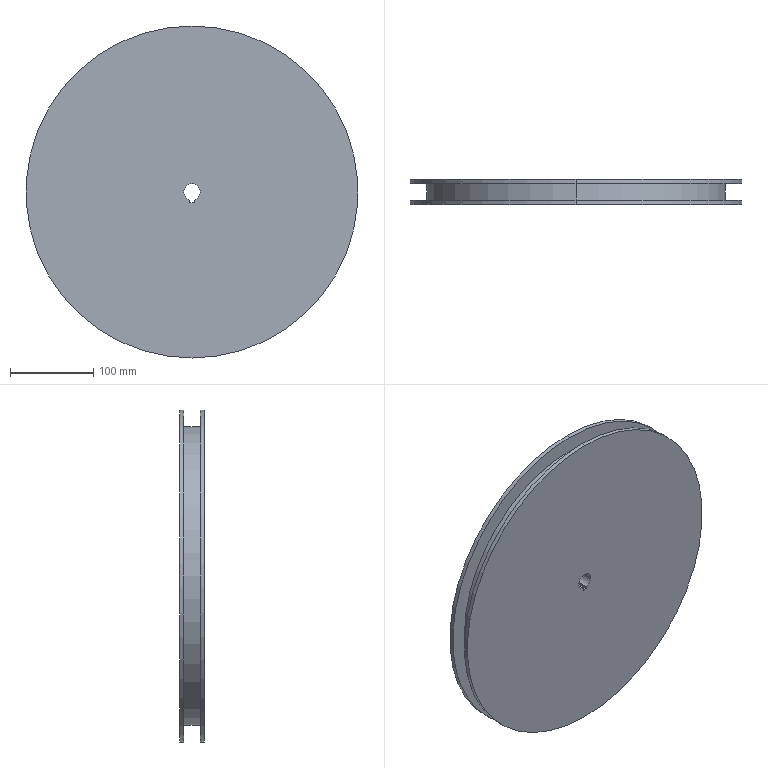Part | SolidWorks | features ICE 1, Revolution 1 | 1 solid | 15 faces | box 400 x 30 x 400 mm | volume 3282546 mm3 | cylinder 8 | plane 7 | commonest cylinder face diameters 400 x4 20 x2 360 x2
STEP:
#1=CARTESIAN_POINT('',(0.,-5.,200.));
#2=VERTEX_POINT('',#1);
#3=CARTESIAN_POINT('',(0.,-5.,-200.));
#4=VERTEX_POINT('',#3);
#5=CARTESIAN_POINT('',(0.,-5.,0.));
#6=DIRECTION('',(0.,1.,0.));
#7=DIRECTION('',(0.,0.,1.));
#8=AXIS2_PLACEMENT_3D('',#5,#6,#7);
#9=CIRCLE('',#8,200.);
#10=EDGE_CURVE('',#2,#4,#9,.T.);
#11=ORIENTED_EDGE('',*,*,#10,.T.);
#12=CARTESIAN_POINT('',(0.,0.,-200.));
#13=VERTEX_POINT('',#12);
#14=CARTESIAN_POINT('',(0.,76.759,-200.));
#15=DIRECTION('',(0.,1.,0.));
#16=VECTOR('',#15,1000.);
#17=LINE('',#14,#16);
#18=EDGE_CURVE('',#4,#13,#17,.T.);
#19=ORIENTED_EDGE('',*,*,#18,.T.);
#20=CARTESIAN_POINT('',(0.,0.,200.));
#21=VERTEX_POINT('',#20);
#22=CARTESIAN_POINT('',(0.,0.,0.));
#23=DIRECTION('',(0.,1.,0.));
#24=DIRECTION('',(0.,0.,1.));
#25=AXIS2_PLACEMENT_3D('',#22,#23,#24);
#26=CIRCLE('',#25,200.);
#27=EDGE_CURVE('',#21,#13,#26,.T.);
#28=ORIENTED_EDGE('',*,*,#27,.F.);
#29=CARTESIAN_POINT('',(0.,76.759,200.));
#30=DIRECTION('',(0.,1.,0.));
#31=VECTOR('',#30,1000.);
#32=LINE('',#29,#31);
#33=EDGE_CURVE('',#2,#21,#32,.T.);
#34=ORIENTED_EDGE('',*,*,#33,.F.);
#35=EDGE_LOOP('',(#11,#19,#28,#34));
#36=FACE_OUTER_BOUND('',#35,.T.);
#37=CARTESIAN_POINT('',(0.,76.759,0.));
#38=DIRECTION('',(0.,1.,0.));
#39=DIRECTION('',(0.,0.,1.));
#40=AXIS2_PLACEMENT_3D('',#37,#38,#39);
#41=CYLINDRICAL_SURFACE('',#40,200.);
#42=ADVANCED_FACE('',(#36),#41,.T.);
#43=CARTESIAN_POINT('',(0.,-25.,180.));
#44=VERTEX_POINT('',#43);
#45=CARTESIAN_POINT('',(0.,-25.,-180.));
#46=VERTEX_POINT('',#45);
#47=CARTESIAN_POINT('',(0.,-25.,0.));
#48=DIRECTION('',(0.,1.,0.));
#49=DIRECTION('',(0.,0.,1.));
#50=AXIS2_PLACEMENT_3D('',#47,#48,#49);
#51=CIRCLE('',#50,180.);
#52=EDGE_CURVE('',#44,#46,#51,.T.);
#53=ORIENTED_EDGE('',*,*,#52,.T.);
#54=CARTESIAN_POINT('',(0.,-5.,-180.));
#55=VERTEX_POINT('',#54);
#56=CARTESIAN_POINT('',(0.,76.759,-180.));
#57=DIRECTION('',(0.,1.,0.));
#58=VECTOR('',#57,1000.);
#59=LINE('',#56,#58);
#60=EDGE_CURVE('',#46,#55,#59,.T.);
#61=ORIENTED_EDGE('',*,*,#60,.T.);
#62=CARTESIAN_POINT('',(0.,-5.,180.));
#63=VERTEX_POINT('',#62);
#64=CARTESIAN_POINT('',(0.,-5.,0.));
#65=DIRECTION('',(0.,1.,0.));
#66=DIRECTION('',(0.,0.,1.));
#67=AXIS2_PLACEMENT_3D('',#64,#65,#66);
#68=CIRCLE('',#67,180.);
#69=EDGE_CURVE('',#63,#55,#68,.T.);
#70=ORIENTED_EDGE('',*,*,#69,.F.);
#71=CARTESIAN_POINT('',(0.,76.759,180.));
#72=DIRECTION('',(0.,1.,0.));
#73=VECTOR('',#72,1000.);
#74=LINE('',#71,#73);
#75=EDGE_CURVE('',#44,#63,#74,.T.);
#76=ORIENTED_EDGE('',*,*,#75,.F.);
#77=EDGE_LOOP('',(#53,#61,#70,#76));
#78=FACE_OUTER_BOUND('',#77,.T.);
#79=CARTESIAN_POINT('',(0.,76.759,0.));
#80=DIRECTION('',(0.,1.,0.));
#81=DIRECTION('',(0.,0.,1.));
#82=AXIS2_PLACEMENT_3D('',#79,#80,#81);
#83=CYLINDRICAL_SURFACE('',#82,180.);
#84=ADVANCED_FACE('',(#78),#83,.T.);
#85=CARTESIAN_POINT('',(0.,-30.,200.));
#86=VERTEX_POINT('',#85);
#87=CARTESIAN_POINT('',(0.,-30.,-200.));
#88=VERTEX_POINT('',#87);
#89=CARTESIAN_POINT('',(0.,-30.,0.));
#90=DIRECTION('',(0.,1.,0.));
#91=DIRECTION('',(0.,0.,1.));
#92=AXIS2_PLACEMENT_3D('',#89,#90,#91);
#93=CIRCLE('',#92,200.);
#94=EDGE_CURVE('',#86,#88,#93,.T.);
#95=ORIENTED_EDGE('',*,*,#94,.T.);
#96=CARTESIAN_POINT('',(0.,-25.,-200.));
#97=VERTEX_POINT('',#96);
#98=CARTESIAN_POINT('',(0.,76.759,-200.));
#99=DIRECTION('',(0.,1.,0.));
#100=VECTOR('',#99,1000.);
#101=LINE('',#98,#100);
#102=EDGE_CURVE('',#88,#97,#101,.T.);
#103=ORIENTED_EDGE('',*,*,#102,.T.);
#104=CARTESIAN_POINT('',(0.,-25.,200.));
#105=VERTEX_POINT('',#104);
#106=CARTESIAN_POINT('',(0.,-25.,0.));
#107=DIRECTION('',(0.,1.,0.));
#108=DIRECTION('',(0.,0.,1.));
#109=AXIS2_PLACEMENT_3D('',#106,#107,#108);
#110=CIRCLE('',#109,200.);
#111=EDGE_CURVE('',#105,#97,#110,.T.);
#112=ORIENTED_EDGE('',*,*,#111,.F.);
#113=CARTESIAN_POINT('',(0.,76.759,200.));
#114=DIRECTION('',(0.,1.,0.));
#115=VECTOR('',#114,1000.);
#116=LINE('',#113,#115);
#117=EDGE_CURVE('',#86,#105,#116,.T.);
#118=ORIENTED_EDGE('',*,*,#117,.F.);
#119=EDGE_LOOP('',(#95,#103,#112,#118));
#120=FACE_OUTER_BOUND('',#119,.T.);
#121=CARTESIAN_POINT('',(0.,76.759,0.));
#122=DIRECTION('',(0.,1.,0.));
#123=DIRECTION('',(0.,0.,1.));
#124=AXIS2_PLACEMENT_3D('',#121,#122,#123);
#125=CYLINDRICAL_SURFACE('',#124,200.);
#126=ADVANCED_FACE('',(#120),#125,.T.);
#127=CARTESIAN_POINT('',(0.,-30.,10.));
#128=VERTEX_POINT('',#127);
#129=CARTESIAN_POINT('',(2.5,-30.,-9.682));
#130=VERTEX_POINT('',#129);
#131=CARTESIAN_POINT('',(0.,-30.,0.));
#132=DIRECTION('',(0.,1.,0.));
#133=DIRECTION('',(0.,0.,1.));
#134=AXIS2_PLACEMENT_3D('',#131,#132,#133);
#135=CIRCLE('',#134,10.);
#136=EDGE_CURVE('',#128,#130,#135,.T.);
#137=ORIENTED_EDGE('',*,*,#136,.F.);
#138=CARTESIAN_POINT('',(0.,0.,10.));
#139=VERTEX_POINT('',#138);
#140=CARTESIAN_POINT('',(0.,76.759,10.));
#141=DIRECTION('',(0.,1.,0.));
#142=VECTOR('',#141,1000.);
#143=LINE('',#140,#142);
#144=EDGE_CURVE('',#128,#139,#143,.T.);
#145=ORIENTED_EDGE('',*,*,#144,.T.);
#146=CARTESIAN_POINT('',(2.5,0.,-9.682));
#147=VERTEX_POINT('',#146);
#148=CARTESIAN_POINT('',(0.,0.,0.));
#149=DIRECTION('',(0.,1.,0.));
#150=DIRECTION('',(0.,0.,1.));
#151=AXIS2_PLACEMENT_3D('',#148,#149,#150);
#152=CIRCLE('',#151,10.);
#153=EDGE_CURVE('',#139,#147,#152,.T.);
#154=ORIENTED_EDGE('',*,*,#153,.T.);
#155=CARTESIAN_POINT('',(2.5,-30.,-9.682));
#156=DIRECTION('',(0.,1.,0.));
#157=VECTOR('',#156,1000.);
#158=LINE('',#155,#157);
#159=EDGE_CURVE('',#130,#147,#158,.T.);
#160=ORIENTED_EDGE('',*,*,#159,.F.);
#161=EDGE_LOOP('',(#137,#145,#154,#160));
#162=FACE_OUTER_BOUND('',#161,.T.);
#163=CARTESIAN_POINT('',(0.,76.759,0.));
#164=DIRECTION('',(0.,1.,0.));
#165=DIRECTION('',(0.,0.,1.));
#166=AXIS2_PLACEMENT_3D('',#163,#164,#165);
#167=CYLINDRICAL_SURFACE('',#166,10.);
#168=ADVANCED_FACE('',(#162),#167,.F.);
#169=CARTESIAN_POINT('',(2.5,0.,-12.682));
#170=VERTEX_POINT('',#169);
#171=CARTESIAN_POINT('',(2.5,0.,-12.682));
#172=DIRECTION('',(0.,0.,-1.));
#173=VECTOR('',#172,1000.);
#174=LINE('',#171,#173);
#175=EDGE_CURVE('',#147,#170,#174,.T.);
#176=ORIENTED_EDGE('',*,*,#175,.F.);
#177=ORIENTED_EDGE('',*,*,#153,.F.);
#178=CARTESIAN_POINT('',(-2.5,0.,-9.682));
#179=VERTEX_POINT('',#178);
#180=CARTESIAN_POINT('',(0.,0.,0.));
#181=DIRECTION('',(0.,1.,0.));
#182=DIRECTION('',(0.,0.,1.));
#183=AXIS2_PLACEMENT_3D('',#180,#181,#182);
#184=CIRCLE('',#183,10.);
#185=EDGE_CURVE('',#179,#139,#184,.T.);
#186=ORIENTED_EDGE('',*,*,#185,.F.);
#187=CARTESIAN_POINT('',(-2.5,0.,-12.682));
#188=VERTEX_POINT('',#187);
#189=CARTESIAN_POINT('',(-2.5,0.,-12.682));
#190=DIRECTION('',(0.,0.,1.));
#191=VECTOR('',#190,1000.);
#192=LINE('',#189,#191);
#193=EDGE_CURVE('',#188,#179,#192,.T.);
#194=ORIENTED_EDGE('',*,*,#193,.F.);
#195=CARTESIAN_POINT('',(-2.5,0.,-12.682));
#196=DIRECTION('',(-1.,0.,0.));
#197=VECTOR('',#196,1000.);
#198=LINE('',#195,#197);
#199=EDGE_CURVE('',#170,#188,#198,.T.);
#200=ORIENTED_EDGE('',*,*,#199,.F.);
#201=EDGE_LOOP('',(#176,#177,#186,#194,#200));
#202=FACE_BOUND('',#201,.T.);
#203=ORIENTED_EDGE('',*,*,#27,.T.);
#204=CARTESIAN_POINT('',(0.,0.,0.));
#205=DIRECTION('',(0.,1.,0.));
#206=DIRECTION('',(0.,0.,1.));
#207=AXIS2_PLACEMENT_3D('',#204,#205,#206);
#208=CIRCLE('',#207,200.);
#209=EDGE_CURVE('',#13,#21,#208,.T.);
#210=ORIENTED_EDGE('',*,*,#209,.T.);
#211=EDGE_LOOP('',(#203,#210));
#212=FACE_OUTER_BOUND('',#211,.T.);
#213=CARTESIAN_POINT('',(-200.,0.,0.));
#214=DIRECTION('',(0.,1.,0.));
#215=DIRECTION('',(0.,0.,1.));
#216=AXIS2_PLACEMENT_3D('',#213,#214,#215);
#217=PLANE('',#216);
#218=ADVANCED_FACE('',(#202,#212),#217,.T.);
#219=ORIENTED_EDGE('',*,*,#144,.F.);
#220=CARTESIAN_POINT('',(-2.5,-30.,-9.682));
#221=VERTEX_POINT('',#220);
#222=CARTESIAN_POINT('',(0.,-30.,0.));
#223=DIRECTION('',(0.,1.,0.));
#224=DIRECTION('',(0.,0.,1.));
#225=AXIS2_PLACEMENT_3D('',#222,#223,#224);
#226=CIRCLE('',#225,10.);
#227=EDGE_CURVE('',#221,#128,#226,.T.);
#228=ORIENTED_EDGE('',*,*,#227,.F.);
#229=CARTESIAN_POINT('',(-2.5,-30.,-9.682));
#230=DIRECTION('',(0.,1.,0.));
#231=VECTOR('',#230,1000.);
#232=LINE('',#229,#231);
#233=EDGE_CURVE('',#221,#179,#232,.T.);
#234=ORIENTED_EDGE('',*,*,#233,.T.);
#235=ORIENTED_EDGE('',*,*,#185,.T.);
#236=EDGE_LOOP('',(#219,#228,#234,#235));
#237=FACE_OUTER_BOUND('',#236,.T.);
#238=CARTESIAN_POINT('',(0.,76.759,0.));
#239=DIRECTION('',(0.,1.,0.));
#240=DIRECTION('',(0.,0.,1.));
#241=AXIS2_PLACEMENT_3D('',#238,#239,#240);
#242=CYLINDRICAL_SURFACE('',#241,10.);
#243=ADVANCED_FACE('',(#237),#242,.F.);
#244=CARTESIAN_POINT('',(2.5,-30.,-12.682));
#245=VERTEX_POINT('',#244);
#246=CARTESIAN_POINT('',(2.5,-30.,-12.682));
#247=DIRECTION('',(0.,0.,-1.));
#248=VECTOR('',#247,1000.);
#249=LINE('',#246,#248);
#250=EDGE_CURVE('',#130,#245,#249,.T.);
#251=ORIENTED_EDGE('',*,*,#250,.T.);
#252=CARTESIAN_POINT('',(-2.5,-30.,-12.682));
#253=VERTEX_POINT('',#252);
#254=CARTESIAN_POINT('',(-2.5,-30.,-12.682));
#255=DIRECTION('',(-1.,0.,0.));
#256=VECTOR('',#255,1000.);
#257=LINE('',#254,#256);
#258=EDGE_CURVE('',#245,#253,#257,.T.);
#259=ORIENTED_EDGE('',*,*,#258,.T.);
#260=CARTESIAN_POINT('',(-2.5,-30.,-12.682));
#261=DIRECTION('',(0.,0.,1.));
#262=VECTOR('',#261,1000.);
#263=LINE('',#260,#262);
#264=EDGE_CURVE('',#253,#221,#263,.T.);
#265=ORIENTED_EDGE('',*,*,#264,.T.);
#266=ORIENTED_EDGE('',*,*,#227,.T.);
#267=ORIENTED_EDGE('',*,*,#136,.T.);
#268=EDGE_LOOP('',(#251,#259,#265,#266,#267));
#269=FACE_BOUND('',#268,.T.);
#270=ORIENTED_EDGE('',*,*,#94,.F.);
#271=CARTESIAN_POINT('',(0.,-30.,0.));
#272=DIRECTION('',(0.,1.,0.));
#273=DIRECTION('',(0.,0.,1.));
#274=AXIS2_PLACEMENT_3D('',#271,#272,#273);
#275=CIRCLE('',#274,200.);
#276=EDGE_CURVE('',#88,#86,#275,.T.);
#277=ORIENTED_EDGE('',*,*,#276,.F.);
#278=EDGE_LOOP('',(#270,#277));
#279=FACE_OUTER_BOUND('',#278,.T.);
#280=CARTESIAN_POINT('',(-10.,-30.,0.));
#281=DIRECTION('',(0.,-1.,0.));
#282=DIRECTION('',(0.,0.,-1.));
#283=AXIS2_PLACEMENT_3D('',#280,#281,#282);
#284=PLANE('',#283);
#285=ADVANCED_FACE('',(#269,#279),#284,.T.);
#286=ORIENTED_EDGE('',*,*,#102,.F.);
#287=ORIENTED_EDGE('',*,*,#276,.T.);
#288=ORIENTED_EDGE('',*,*,#117,.T.);
#289=CARTESIAN_POINT('',(0.,-25.,0.));
#290=DIRECTION('',(0.,1.,0.));
#291=DIRECTION('',(0.,0.,1.));
#292=AXIS2_PLACEMENT_3D('',#289,#290,#291);
#293=CIRCLE('',#292,200.);
#294=EDGE_CURVE('',#97,#105,#293,.T.);
#295=ORIENTED_EDGE('',*,*,#294,.F.);
#296=EDGE_LOOP('',(#286,#287,#288,#295));
#297=FACE_OUTER_BOUND('',#296,.T.);
#298=CARTESIAN_POINT('',(0.,76.759,0.));
#299=DIRECTION('',(0.,1.,0.));
#300=DIRECTION('',(0.,0.,1.));
#301=AXIS2_PLACEMENT_3D('',#298,#299,#300);
#302=CYLINDRICAL_SURFACE('',#301,200.);
#303=ADVANCED_FACE('',(#297),#302,.T.);
#304=ORIENTED_EDGE('',*,*,#111,.T.);
#305=ORIENTED_EDGE('',*,*,#294,.T.);
#306=EDGE_LOOP('',(#304,#305));
#307=FACE_OUTER_BOUND('',#306,.T.);
#308=ORIENTED_EDGE('',*,*,#52,.F.);
#309=CARTESIAN_POINT('',(0.,-25.,0.));
#310=DIRECTION('',(0.,1.,0.));
#311=DIRECTION('',(0.,0.,1.));
#312=AXIS2_PLACEMENT_3D('',#309,#310,#311);
#313=CIRCLE('',#312,180.);
#314=EDGE_CURVE('',#46,#44,#313,.T.);
#315=ORIENTED_EDGE('',*,*,#314,.F.);
#316=EDGE_LOOP('',(#308,#315));
#317=FACE_BOUND('',#316,.T.);
#318=CARTESIAN_POINT('',(-200.,-25.,0.));
#319=DIRECTION('',(0.,1.,0.));
#320=DIRECTION('',(0.,0.,1.));
#321=AXIS2_PLACEMENT_3D('',#318,#319,#320);
#322=PLANE('',#321);
#323=ADVANCED_FACE('',(#307,#317),#322,.T.);
#324=ORIENTED_EDGE('',*,*,#60,.F.);
#325=ORIENTED_EDGE('',*,*,#314,.T.);
#326=ORIENTED_EDGE('',*,*,#75,.T.);
#327=CARTESIAN_POINT('',(0.,-5.,0.));
#328=DIRECTION('',(0.,1.,0.));
#329=DIRECTION('',(0.,0.,1.));
#330=AXIS2_PLACEMENT_3D('',#327,#328,#329);
#331=CIRCLE('',#330,180.);
#332=EDGE_CURVE('',#55,#63,#331,.T.);
#333=ORIENTED_EDGE('',*,*,#332,.F.);
#334=EDGE_LOOP('',(#324,#325,#326,#333));
#335=FACE_OUTER_BOUND('',#334,.T.);
#336=CARTESIAN_POINT('',(0.,76.759,0.));
#337=DIRECTION('',(0.,1.,0.));
#338=DIRECTION('',(0.,0.,1.));
#339=AXIS2_PLACEMENT_3D('',#336,#337,#338);
#340=CYLINDRICAL_SURFACE('',#339,180.);
#341=ADVANCED_FACE('',(#335),#340,.T.);
#342=ORIENTED_EDGE('',*,*,#69,.T.);
#343=ORIENTED_EDGE('',*,*,#332,.T.);
#344=EDGE_LOOP('',(#342,#343));
#345=FACE_BOUND('',#344,.T.);
#346=ORIENTED_EDGE('',*,*,#10,.F.);
#347=CARTESIAN_POINT('',(0.,-5.,0.));
#348=DIRECTION('',(0.,1.,0.));
#349=DIRECTION('',(0.,0.,1.));
#350=AXIS2_PLACEMENT_3D('',#347,#348,#349);
#351=CIRCLE('',#350,200.);
#352=EDGE_CURVE('',#4,#2,#351,.T.);
#353=ORIENTED_EDGE('',*,*,#352,.F.);
#354=EDGE_LOOP('',(#346,#353));
#355=FACE_OUTER_BOUND('',#354,.T.);
#356=CARTESIAN_POINT('',(-180.,-5.,0.));
#357=DIRECTION('',(0.,-1.,0.));
#358=DIRECTION('',(0.,0.,-1.));
#359=AXIS2_PLACEMENT_3D('',#356,#357,#358);
#360=PLANE('',#359);
#361=ADVANCED_FACE('',(#345,#355),#360,.T.);
#362=ORIENTED_EDGE('',*,*,#18,.F.);
#363=ORIENTED_EDGE('',*,*,#352,.T.);
#364=ORIENTED_EDGE('',*,*,#33,.T.);
#365=ORIENTED_EDGE('',*,*,#209,.F.);
#366=EDGE_LOOP('',(#362,#363,#364,#365));
#367=FACE_OUTER_BOUND('',#366,.T.);
#368=CARTESIAN_POINT('',(0.,76.759,0.));
#369=DIRECTION('',(0.,1.,0.));
#370=DIRECTION('',(0.,0.,1.));
#371=AXIS2_PLACEMENT_3D('',#368,#369,#370);
#372=CYLINDRICAL_SURFACE('',#371,200.);
#373=ADVANCED_FACE('',(#367),#372,.T.);
#374=ORIENTED_EDGE('',*,*,#199,.T.);
#375=CARTESIAN_POINT('',(-2.5,-30.,-12.682));
#376=DIRECTION('',(0.,1.,0.));
#377=VECTOR('',#376,1000.);
#378=LINE('',#375,#377);
#379=EDGE_CURVE('',#253,#188,#378,.T.);
#380=ORIENTED_EDGE('',*,*,#379,.F.);
#381=ORIENTED_EDGE('',*,*,#258,.F.);
#382=CARTESIAN_POINT('',(2.5,-30.,-12.682));
#383=DIRECTION('',(0.,1.,0.));
#384=VECTOR('',#383,1000.);
#385=LINE('',#382,#384);
#386=EDGE_CURVE('',#245,#170,#385,.T.);
#387=ORIENTED_EDGE('',*,*,#386,.T.);
#388=EDGE_LOOP('',(#374,#380,#381,#387));
#389=FACE_OUTER_BOUND('',#388,.T.);
#390=CARTESIAN_POINT('',(-2.5,-30.,-12.682));
#391=DIRECTION('',(0.,0.,-1.));
#392=DIRECTION('',(-1.,0.,0.));
#393=AXIS2_PLACEMENT_3D('',#390,#391,#392);
#394=PLANE('',#393);
#395=ADVANCED_FACE('',(#389),#394,.F.);
#396=ORIENTED_EDGE('',*,*,#175,.T.);
#397=ORIENTED_EDGE('',*,*,#386,.F.);
#398=ORIENTED_EDGE('',*,*,#250,.F.);
#399=ORIENTED_EDGE('',*,*,#159,.T.);
#400=EDGE_LOOP('',(#396,#397,#398,#399));
#401=FACE_OUTER_BOUND('',#400,.T.);
#402=CARTESIAN_POINT('',(2.5,-30.,-12.682));
#403=DIRECTION('',(1.,0.,0.));
#404=DIRECTION('',(0.,0.,-1.));
#405=AXIS2_PLACEMENT_3D('',#402,#403,#404);
#406=PLANE('',#405);
#407=ADVANCED_FACE('',(#401),#406,.F.);
#408=ORIENTED_EDGE('',*,*,#193,.T.);
#409=ORIENTED_EDGE('',*,*,#233,.F.);
#410=ORIENTED_EDGE('',*,*,#264,.F.);
#411=ORIENTED_EDGE('',*,*,#379,.T.);
#412=EDGE_LOOP('',(#408,#409,#410,#411));
#413=FACE_OUTER_BOUND('',#412,.T.);
#414=CARTESIAN_POINT('',(-2.5,-30.,-12.682));
#415=DIRECTION('',(-1.,0.,0.));
#416=DIRECTION('',(0.,0.,1.));
#417=AXIS2_PLACEMENT_3D('',#414,#415,#416);
#418=PLANE('',#417);
#419=ADVANCED_FACE('',(#413),#418,.F.);
#420=CLOSED_SHELL('',(#42,#84,#126,#168,#218,#243,#285,#303,#323,#341,#361,#373,#395,#407,#419));
#421=MANIFOLD_SOLID_BREP('',#420);
#422=CARTESIAN_POINT('',(0.,0.,0.));
#423=DIRECTION('',(0.,0.,1.));
#424=DIRECTION('',(1.,0.,0.));
#425=AXIS2_PLACEMENT_3D('',#422,#423,#424);
#426=(LENGTH_UNIT()NAMED_UNIT(*)SI_UNIT(.MILLI.,.METRE.));
#427=UNCERTAINTY_MEASURE_WITH_UNIT(LENGTH_MEASURE(0.00001),#426,'','');
#428=(NAMED_UNIT(*)PLANE_ANGLE_UNIT()SI_UNIT($,.RADIAN.));
#429=(NAMED_UNIT(*)SI_UNIT($,.STERADIAN.)SOLID_ANGLE_UNIT());
#430=(GEOMETRIC_REPRESENTATION_CONTEXT(3)GLOBAL_UNCERTAINTY_ASSIGNED_CONTEXT((#427))GLOBAL_UNIT_ASSIGNED_CONTEXT((#426,#428,#429))REPRESENTATION_CONTEXT('',''));
#431=ADVANCED_BREP_SHAPE_REPRESENTATION('',(#421,#425),#430);